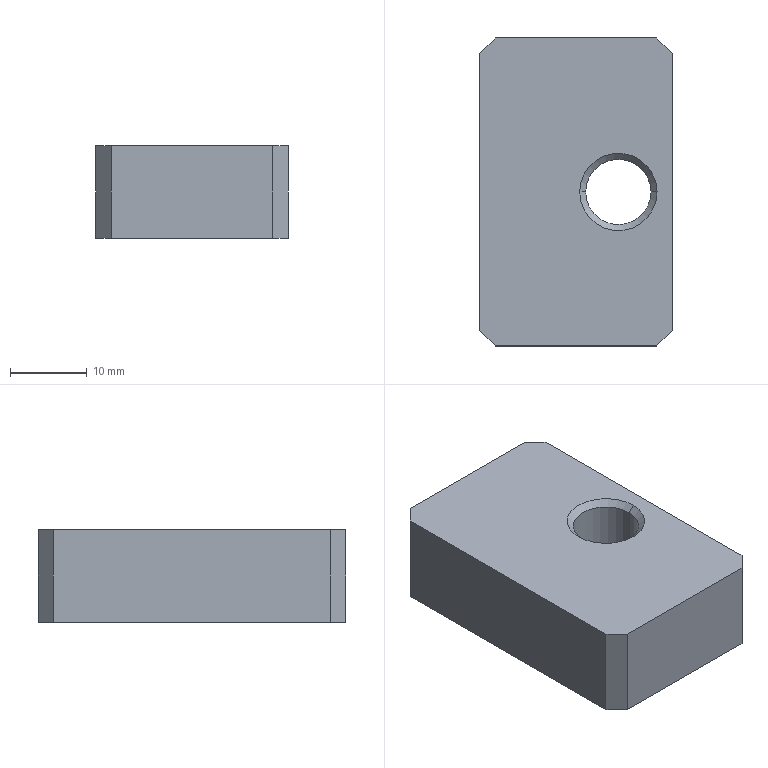Part | STEP file | 001-004-Feeding mechanism hydraulic buffer mounting plate | 1 solid | 14 faces | box 25 x 40 x 12 mm | volume 11215 mm3 | plane 10 | cone 2 | cylinder 2 | commonest cylinder face diameters 8.5 x2
STEP:
#1=CARTESIAN_POINT('',(0.,0.,0.));
#2=DIRECTION('',(0.,0.,1.));
#3=DIRECTION('',(1.,0.,0.));
#4=AXIS2_PLACEMENT_3D('',#1,#2,#3);
#5=CARTESIAN_POINT('',(9.75,0.,11.225));
#6=VERTEX_POINT('',#5);
#7=CARTESIAN_POINT('',(10.525,0.,12.));
#8=VERTEX_POINT('',#7);
#9=CARTESIAN_POINT('',(10.525,0.,12.));
#10=DIRECTION('',(0.7071,0.,0.7071));
#11=VECTOR('',#10,1.);
#12=LINE('',#9,#11);
#13=CARTESIAN_POINT('',(5.5,0.,12.));
#14=DIRECTION('',(0.,0.,1.));
#15=DIRECTION('',(1.,0.,0.));
#16=AXIS2_PLACEMENT_3D('',#13,#14,#15);
#17=CONICAL_SURFACE('',#16,5.025,0.7854);
#18=CARTESIAN_POINT('',(6.283,0.));
#19=DIRECTION('',(0.,1.));
#20=VECTOR('',#19,1.);
#21=LINE('',#18,#20);
#22=(GEOMETRIC_REPRESENTATION_CONTEXT(2)PARAMETRIC_REPRESENTATION_CONTEXT()REPRESENTATION_CONTEXT('',''));
#23=DEFINITIONAL_REPRESENTATION('',(#21),#22);
#24=PCURVE('',#17,#23);
#25=CARTESIAN_POINT('',(5.5,0.,12.));
#26=DIRECTION('',(0.,0.,1.));
#27=DIRECTION('',(1.,0.,0.));
#28=AXIS2_PLACEMENT_3D('',#25,#26,#27);
#29=CONICAL_SURFACE('',#28,5.025,0.7854);
#30=CARTESIAN_POINT('',(0.,0.));
#31=DIRECTION('',(0.,1.));
#32=VECTOR('',#31,1.);
#33=LINE('',#30,#32);
#34=(GEOMETRIC_REPRESENTATION_CONTEXT(2)PARAMETRIC_REPRESENTATION_CONTEXT()REPRESENTATION_CONTEXT('',''));
#35=DEFINITIONAL_REPRESENTATION('',(#33),#34);
#36=PCURVE('',#29,#35);
#37=SURFACE_CURVE('',#12,(#24,#36),.PCURVE_S1.);
#38=EDGE_CURVE('',#6,#8,#37,.T.);
#39=ORIENTED_EDGE('',*,*,#38,.T.);
#40=CARTESIAN_POINT('',(0.475,0.,12.));
#41=VERTEX_POINT('',#40);
#42=CARTESIAN_POINT('',(5.5,0.,12.));
#43=DIRECTION('',(0.,0.,1.));
#44=DIRECTION('',(1.,0.,0.));
#45=AXIS2_PLACEMENT_3D('',#42,#43,#44);
#46=CIRCLE('',#45,5.025);
#47=CARTESIAN_POINT('',(0.,0.));
#48=DIRECTION('',(1.,0.));
#49=VECTOR('',#48,1.);
#50=LINE('',#47,#49);
#51=(GEOMETRIC_REPRESENTATION_CONTEXT(2)PARAMETRIC_REPRESENTATION_CONTEXT()REPRESENTATION_CONTEXT('',''));
#52=DEFINITIONAL_REPRESENTATION('',(#50),#51);
#53=PCURVE('',#17,#52);
#54=CARTESIAN_POINT('',(0.,0.,12.));
#55=DIRECTION('',(0.,0.,-1.));
#56=DIRECTION('',(-1.,0.,0.));
#57=AXIS2_PLACEMENT_3D('',#54,#55,#56);
#58=PLANE('',#57);
#59=CARTESIAN_POINT('',(-10.525,0.));
#60=CARTESIAN_POINT('',(-10.525,8.704));
#61=CARTESIAN_POINT('',(-2.988,4.352));
#62=CARTESIAN_POINT('',(4.55,0.));
#63=CARTESIAN_POINT('',(-2.988,-4.352));
#64=CARTESIAN_POINT('',(-10.525,-8.704));
#65=CARTESIAN_POINT('',(-10.525,0.));
#66=(BOUNDED_CURVE()B_SPLINE_CURVE(2,(#59,#60,#61,#62,#63,#64,#65),.UNSPECIFIED.,.T.,.F.)B_SPLINE_CURVE_WITH_KNOTS((1,2,2,2,2,1),(-2.094,0.,2.094,4.189,6.283,8.378),.UNSPECIFIED.)CURVE()GEOMETRIC_REPRESENTATION_ITEM()RATIONAL_B_SPLINE_CURVE((1.,0.5,1.,0.5,1.,0.5,1.))REPRESENTATION_ITEM(''));
#67=(GEOMETRIC_REPRESENTATION_CONTEXT(2)PARAMETRIC_REPRESENTATION_CONTEXT()REPRESENTATION_CONTEXT('',''));
#68=DEFINITIONAL_REPRESENTATION('',(#66),#67);
#69=PCURVE('',#58,#68);
#70=SURFACE_CURVE('',#46,(#53,#69),.PCURVE_S1.);
#71=EDGE_CURVE('',#41,#8,#70,.T.);
#72=ORIENTED_EDGE('',*,*,#71,.F.);
#73=CARTESIAN_POINT('',(1.25,0.,11.225));
#74=VERTEX_POINT('',#73);
#75=CARTESIAN_POINT('',(0.475,0.,12.));
#76=DIRECTION('',(-0.7071,0.,0.7071));
#77=VECTOR('',#76,1.);
#78=LINE('',#75,#77);
#79=CARTESIAN_POINT('',(3.142,0.));
#80=DIRECTION('',(0.,1.));
#81=VECTOR('',#80,1.);
#82=LINE('',#79,#81);
#83=(GEOMETRIC_REPRESENTATION_CONTEXT(2)PARAMETRIC_REPRESENTATION_CONTEXT()REPRESENTATION_CONTEXT('',''));
#84=DEFINITIONAL_REPRESENTATION('',(#82),#83);
#85=PCURVE('',#17,#84);
#86=CARTESIAN_POINT('',(3.142,0.));
#87=DIRECTION('',(0.,1.));
#88=VECTOR('',#87,1.);
#89=LINE('',#86,#88);
#90=(GEOMETRIC_REPRESENTATION_CONTEXT(2)PARAMETRIC_REPRESENTATION_CONTEXT()REPRESENTATION_CONTEXT('',''));
#91=DEFINITIONAL_REPRESENTATION('',(#89),#90);
#92=PCURVE('',#29,#91);
#93=SURFACE_CURVE('',#78,(#85,#92),.PCURVE_S1.);
#94=EDGE_CURVE('',#74,#41,#93,.T.);
#95=ORIENTED_EDGE('',*,*,#94,.F.);
#96=CARTESIAN_POINT('',(5.5,0.,11.225));
#97=DIRECTION('',(0.,0.,1.));
#98=DIRECTION('',(1.,0.,0.));
#99=AXIS2_PLACEMENT_3D('',#96,#97,#98);
#100=CIRCLE('',#99,4.25);
#101=CARTESIAN_POINT('',(0.,-0.775));
#102=DIRECTION('',(1.,0.));
#103=VECTOR('',#102,1.);
#104=LINE('',#101,#103);
#105=(GEOMETRIC_REPRESENTATION_CONTEXT(2)PARAMETRIC_REPRESENTATION_CONTEXT()REPRESENTATION_CONTEXT('',''));
#106=DEFINITIONAL_REPRESENTATION('',(#104),#105);
#107=PCURVE('',#17,#106);
#108=CARTESIAN_POINT('',(5.5,0.,12.));
#109=DIRECTION('',(0.,0.,1.));
#110=DIRECTION('',(1.,0.,0.));
#111=AXIS2_PLACEMENT_3D('',#108,#109,#110);
#112=CYLINDRICAL_SURFACE('',#111,4.25);
#113=CARTESIAN_POINT('',(0.,-0.775));
#114=DIRECTION('',(1.,0.));
#115=VECTOR('',#114,1.);
#116=LINE('',#113,#115);
#117=(GEOMETRIC_REPRESENTATION_CONTEXT(2)PARAMETRIC_REPRESENTATION_CONTEXT()REPRESENTATION_CONTEXT('',''));
#118=DEFINITIONAL_REPRESENTATION('',(#116),#117);
#119=PCURVE('',#112,#118);
#120=SURFACE_CURVE('',#100,(#107,#119),.PCURVE_S1.);
#121=EDGE_CURVE('',#74,#6,#120,.T.);
#122=ORIENTED_EDGE('',*,*,#121,.T.);
#123=EDGE_LOOP('',(#39,#72,#95,#122));
#124=FACE_BOUND('',#123,.F.);
#125=ADVANCED_FACE('',(#124),#17,.F.);
#126=CARTESIAN_POINT('',(9.75,0.,0.));
#127=VERTEX_POINT('',#126);
#128=CARTESIAN_POINT('',(9.75,0.,12.));
#129=DIRECTION('',(0.,0.,1.));
#130=VECTOR('',#129,1.);
#131=LINE('',#128,#130);
#132=CARTESIAN_POINT('',(6.283,0.));
#133=DIRECTION('',(0.,1.));
#134=VECTOR('',#133,1.);
#135=LINE('',#132,#134);
#136=(GEOMETRIC_REPRESENTATION_CONTEXT(2)PARAMETRIC_REPRESENTATION_CONTEXT()REPRESENTATION_CONTEXT('',''));
#137=DEFINITIONAL_REPRESENTATION('',(#135),#136);
#138=PCURVE('',#112,#137);
#139=CARTESIAN_POINT('',(5.5,0.,12.));
#140=DIRECTION('',(0.,0.,1.));
#141=DIRECTION('',(1.,0.,0.));
#142=AXIS2_PLACEMENT_3D('',#139,#140,#141);
#143=CYLINDRICAL_SURFACE('',#142,4.25);
#144=CARTESIAN_POINT('',(0.,0.));
#145=DIRECTION('',(0.,1.));
#146=VECTOR('',#145,1.);
#147=LINE('',#144,#146);
#148=(GEOMETRIC_REPRESENTATION_CONTEXT(2)PARAMETRIC_REPRESENTATION_CONTEXT()REPRESENTATION_CONTEXT('',''));
#149=DEFINITIONAL_REPRESENTATION('',(#147),#148);
#150=PCURVE('',#143,#149);
#151=SURFACE_CURVE('',#131,(#138,#150),.PCURVE_S1.);
#152=EDGE_CURVE('',#127,#6,#151,.T.);
#153=ORIENTED_EDGE('',*,*,#152,.T.);
#154=ORIENTED_EDGE('',*,*,#121,.F.);
#155=CARTESIAN_POINT('',(1.25,0.,0.));
#156=VERTEX_POINT('',#155);
#157=CARTESIAN_POINT('',(1.25,0.,12.));
#158=DIRECTION('',(0.,0.,1.));
#159=VECTOR('',#158,1.);
#160=LINE('',#157,#159);
#161=CARTESIAN_POINT('',(3.142,0.));
#162=DIRECTION('',(0.,1.));
#163=VECTOR('',#162,1.);
#164=LINE('',#161,#163);
#165=(GEOMETRIC_REPRESENTATION_CONTEXT(2)PARAMETRIC_REPRESENTATION_CONTEXT()REPRESENTATION_CONTEXT('',''));
#166=DEFINITIONAL_REPRESENTATION('',(#164),#165);
#167=PCURVE('',#112,#166);
#168=CARTESIAN_POINT('',(3.142,0.));
#169=DIRECTION('',(0.,1.));
#170=VECTOR('',#169,1.);
#171=LINE('',#168,#170);
#172=(GEOMETRIC_REPRESENTATION_CONTEXT(2)PARAMETRIC_REPRESENTATION_CONTEXT()REPRESENTATION_CONTEXT('',''));
#173=DEFINITIONAL_REPRESENTATION('',(#171),#172);
#174=PCURVE('',#143,#173);
#175=SURFACE_CURVE('',#160,(#167,#174),.PCURVE_S1.);
#176=EDGE_CURVE('',#156,#74,#175,.T.);
#177=ORIENTED_EDGE('',*,*,#176,.F.);
#178=CARTESIAN_POINT('',(5.5,0.,0.));
#179=DIRECTION('',(0.,0.,1.));
#180=DIRECTION('',(1.,0.,0.));
#181=AXIS2_PLACEMENT_3D('',#178,#179,#180);
#182=CIRCLE('',#181,4.25);
#183=CARTESIAN_POINT('',(0.,-12.));
#184=DIRECTION('',(1.,0.));
#185=VECTOR('',#184,1.);
#186=LINE('',#183,#185);
#187=(GEOMETRIC_REPRESENTATION_CONTEXT(2)PARAMETRIC_REPRESENTATION_CONTEXT()REPRESENTATION_CONTEXT('',''));
#188=DEFINITIONAL_REPRESENTATION('',(#186),#187);
#189=PCURVE('',#112,#188);
#190=CARTESIAN_POINT('',(0.,0.,0.));
#191=DIRECTION('',(0.,0.,-1.));
#192=DIRECTION('',(-1.,0.,0.));
#193=AXIS2_PLACEMENT_3D('',#190,#191,#192);
#194=PLANE('',#193);
#195=CARTESIAN_POINT('',(-9.75,0.));
#196=CARTESIAN_POINT('',(-9.75,7.361));
#197=CARTESIAN_POINT('',(-3.375,3.681));
#198=CARTESIAN_POINT('',(3.,0.));
#199=CARTESIAN_POINT('',(-3.375,-3.681));
#200=CARTESIAN_POINT('',(-9.75,-7.361));
#201=CARTESIAN_POINT('',(-9.75,0.));
#202=(BOUNDED_CURVE()B_SPLINE_CURVE(2,(#195,#196,#197,#198,#199,#200,#201),.UNSPECIFIED.,.T.,.F.)B_SPLINE_CURVE_WITH_KNOTS((1,2,2,2,2,1),(-2.094,0.,2.094,4.189,6.283,8.378),.UNSPECIFIED.)CURVE()GEOMETRIC_REPRESENTATION_ITEM()RATIONAL_B_SPLINE_CURVE((1.,0.5,1.,0.5,1.,0.5,1.))REPRESENTATION_ITEM(''));
#203=(GEOMETRIC_REPRESENTATION_CONTEXT(2)PARAMETRIC_REPRESENTATION_CONTEXT()REPRESENTATION_CONTEXT('',''));
#204=DEFINITIONAL_REPRESENTATION('',(#202),#203);
#205=PCURVE('',#194,#204);
#206=SURFACE_CURVE('',#182,(#189,#205),.PCURVE_S1.);
#207=EDGE_CURVE('',#156,#127,#206,.T.);
#208=ORIENTED_EDGE('',*,*,#207,.T.);
#209=EDGE_LOOP('',(#153,#154,#177,#208));
#210=FACE_BOUND('',#209,.F.);
#211=ADVANCED_FACE('',(#210),#112,.F.);
#212=CARTESIAN_POINT('',(12.5,-18.,12.));
#213=VERTEX_POINT('',#212);
#214=CARTESIAN_POINT('',(12.5,18.,12.));
#215=VERTEX_POINT('',#214);
#216=CARTESIAN_POINT('',(12.5,-20.,12.));
#217=DIRECTION('',(0.,1.,0.));
#218=VECTOR('',#217,1.);
#219=LINE('',#216,#218);
#220=CARTESIAN_POINT('',(12.5,-20.,12.));
#221=DIRECTION('',(-1.,0.,0.));
#222=DIRECTION('',(0.,0.,1.));
#223=AXIS2_PLACEMENT_3D('',#220,#221,#222);
#224=PLANE('',#223);
#225=CARTESIAN_POINT('',(0.,0.));
#226=DIRECTION('',(0.,1.));
#227=VECTOR('',#226,1.);
#228=LINE('',#225,#227);
#229=(GEOMETRIC_REPRESENTATION_CONTEXT(2)PARAMETRIC_REPRESENTATION_CONTEXT()REPRESENTATION_CONTEXT('',''));
#230=DEFINITIONAL_REPRESENTATION('',(#228),#229);
#231=PCURVE('',#224,#230);
#232=CARTESIAN_POINT('',(-12.5,-20.));
#233=DIRECTION('',(0.,1.));
#234=VECTOR('',#233,1.);
#235=LINE('',#232,#234);
#236=(GEOMETRIC_REPRESENTATION_CONTEXT(2)PARAMETRIC_REPRESENTATION_CONTEXT()REPRESENTATION_CONTEXT('',''));
#237=DEFINITIONAL_REPRESENTATION('',(#235),#236);
#238=PCURVE('',#58,#237);
#239=SURFACE_CURVE('',#219,(#231,#238),.PCURVE_S1.);
#240=EDGE_CURVE('',#213,#215,#239,.T.);
#241=ORIENTED_EDGE('',*,*,#240,.F.);
#242=CARTESIAN_POINT('',(12.5,-18.,0.));
#243=VERTEX_POINT('',#242);
#244=CARTESIAN_POINT('',(12.5,-18.,12.));
#245=DIRECTION('',(0.,0.,-1.));
#246=VECTOR('',#245,1.);
#247=LINE('',#244,#246);
#248=CARTESIAN_POINT('',(0.,2.));
#249=DIRECTION('',(-1.,0.));
#250=VECTOR('',#249,1.);
#251=LINE('',#248,#250);
#252=(GEOMETRIC_REPRESENTATION_CONTEXT(2)PARAMETRIC_REPRESENTATION_CONTEXT()REPRESENTATION_CONTEXT('',''));
#253=DEFINITIONAL_REPRESENTATION('',(#251),#252);
#254=PCURVE('',#224,#253);
#255=CARTESIAN_POINT('',(12.5,-18.,12.));
#256=DIRECTION('',(-0.7071,0.7071,0.));
#257=DIRECTION('',(0.,0.,-1.));
#258=AXIS2_PLACEMENT_3D('',#255,#256,#257);
#259=PLANE('',#258);
#260=CARTESIAN_POINT('',(0.,0.));
#261=DIRECTION('',(1.,0.));
#262=VECTOR('',#261,1.);
#263=LINE('',#260,#262);
#264=(GEOMETRIC_REPRESENTATION_CONTEXT(2)PARAMETRIC_REPRESENTATION_CONTEXT()REPRESENTATION_CONTEXT('',''));
#265=DEFINITIONAL_REPRESENTATION('',(#263),#264);
#266=PCURVE('',#259,#265);
#267=SURFACE_CURVE('',#247,(#254,#266),.PCURVE_S1.);
#268=EDGE_CURVE('',#213,#243,#267,.T.);
#269=ORIENTED_EDGE('',*,*,#268,.T.);
#270=CARTESIAN_POINT('',(12.5,18.,0.));
#271=VERTEX_POINT('',#270);
#272=CARTESIAN_POINT('',(12.5,-20.,0.));
#273=DIRECTION('',(0.,1.,0.));
#274=VECTOR('',#273,1.);
#275=LINE('',#272,#274);
#276=CARTESIAN_POINT('',(-12.,0.));
#277=DIRECTION('',(0.,1.));
#278=VECTOR('',#277,1.);
#279=LINE('',#276,#278);
#280=(GEOMETRIC_REPRESENTATION_CONTEXT(2)PARAMETRIC_REPRESENTATION_CONTEXT()REPRESENTATION_CONTEXT('',''));
#281=DEFINITIONAL_REPRESENTATION('',(#279),#280);
#282=PCURVE('',#224,#281);
#283=CARTESIAN_POINT('',(-12.5,-20.));
#284=DIRECTION('',(0.,1.));
#285=VECTOR('',#284,1.);
#286=LINE('',#283,#285);
#287=(GEOMETRIC_REPRESENTATION_CONTEXT(2)PARAMETRIC_REPRESENTATION_CONTEXT()REPRESENTATION_CONTEXT('',''));
#288=DEFINITIONAL_REPRESENTATION('',(#286),#287);
#289=PCURVE('',#194,#288);
#290=SURFACE_CURVE('',#275,(#282,#289),.PCURVE_S1.);
#291=EDGE_CURVE('',#243,#271,#290,.T.);
#292=ORIENTED_EDGE('',*,*,#291,.T.);
#293=CARTESIAN_POINT('',(12.5,18.,12.));
#294=DIRECTION('',(0.,0.,1.));
#295=VECTOR('',#294,1.);
#296=LINE('',#293,#295);
#297=CARTESIAN_POINT('',(0.,38.));
#298=DIRECTION('',(1.,0.));
#299=VECTOR('',#298,1.);
#300=LINE('',#297,#299);
#301=(GEOMETRIC_REPRESENTATION_CONTEXT(2)PARAMETRIC_REPRESENTATION_CONTEXT()REPRESENTATION_CONTEXT('',''));
#302=DEFINITIONAL_REPRESENTATION('',(#300),#301);
#303=PCURVE('',#224,#302);
#304=CARTESIAN_POINT('',(10.5,20.,12.));
#305=DIRECTION('',(-0.7071,-0.7071,0.));
#306=DIRECTION('',(0.,0.,-1.));
#307=AXIS2_PLACEMENT_3D('',#304,#305,#306);
#308=PLANE('',#307);
#309=CARTESIAN_POINT('',(0.,2.828));
#310=DIRECTION('',(-1.,0.));
#311=VECTOR('',#310,1.);
#312=LINE('',#309,#311);
#313=(GEOMETRIC_REPRESENTATION_CONTEXT(2)PARAMETRIC_REPRESENTATION_CONTEXT()REPRESENTATION_CONTEXT('',''));
#314=DEFINITIONAL_REPRESENTATION('',(#312),#313);
#315=PCURVE('',#308,#314);
#316=SURFACE_CURVE('',#296,(#303,#315),.PCURVE_S1.);
#317=EDGE_CURVE('',#271,#215,#316,.T.);
#318=ORIENTED_EDGE('',*,*,#317,.T.);
#319=EDGE_LOOP('',(#241,#269,#292,#318));
#320=FACE_BOUND('',#319,.T.);
#321=ADVANCED_FACE('',(#320),#224,.F.);
#322=CARTESIAN_POINT('',(10.5,20.,0.));
#323=VERTEX_POINT('',#322);
#324=CARTESIAN_POINT('',(-10.5,20.,0.));
#325=VERTEX_POINT('',#324);
#326=CARTESIAN_POINT('',(-12.5,20.,0.));
#327=DIRECTION('',(-1.,0.,0.));
#328=VECTOR('',#327,1.);
#329=LINE('',#326,#328);
#330=CARTESIAN_POINT('',(-12.5,20.,12.));
#331=DIRECTION('',(0.,-1.,0.));
#332=DIRECTION('',(0.,0.,-1.));
#333=AXIS2_PLACEMENT_3D('',#330,#331,#332);
#334=PLANE('',#333);
#335=CARTESIAN_POINT('',(12.,0.));
#336=DIRECTION('',(0.,-1.));
#337=VECTOR('',#336,1.);
#338=LINE('',#335,#337);
#339=(GEOMETRIC_REPRESENTATION_CONTEXT(2)PARAMETRIC_REPRESENTATION_CONTEXT()REPRESENTATION_CONTEXT('',''));
#340=DEFINITIONAL_REPRESENTATION('',(#338),#339);
#341=PCURVE('',#334,#340);
#342=CARTESIAN_POINT('',(12.5,20.));
#343=DIRECTION('',(1.,0.));
#344=VECTOR('',#343,1.);
#345=LINE('',#342,#344);
#346=(GEOMETRIC_REPRESENTATION_CONTEXT(2)PARAMETRIC_REPRESENTATION_CONTEXT()REPRESENTATION_CONTEXT('',''));
#347=DEFINITIONAL_REPRESENTATION('',(#345),#346);
#348=PCURVE('',#194,#347);
#349=SURFACE_CURVE('',#329,(#341,#348),.PCURVE_S1.);
#350=EDGE_CURVE('',#323,#325,#349,.T.);
#351=ORIENTED_EDGE('',*,*,#350,.T.);
#352=CARTESIAN_POINT('',(-10.5,20.,12.));
#353=VERTEX_POINT('',#352);
#354=CARTESIAN_POINT('',(-10.5,20.,12.));
#355=DIRECTION('',(0.,0.,1.));
#356=VECTOR('',#355,1.);
#357=LINE('',#354,#356);
#358=CARTESIAN_POINT('',(0.,2.));
#359=DIRECTION('',(-1.,0.));
#360=VECTOR('',#359,1.);
#361=LINE('',#358,#360);
#362=(GEOMETRIC_REPRESENTATION_CONTEXT(2)PARAMETRIC_REPRESENTATION_CONTEXT()REPRESENTATION_CONTEXT('',''));
#363=DEFINITIONAL_REPRESENTATION('',(#361),#362);
#364=PCURVE('',#334,#363);
#365=CARTESIAN_POINT('',(-12.5,18.,12.));
#366=DIRECTION('',(0.7071,-0.7071,0.));
#367=DIRECTION('',(0.,0.,-1.));
#368=AXIS2_PLACEMENT_3D('',#365,#366,#367);
#369=PLANE('',#368);
#370=CARTESIAN_POINT('',(0.,2.828));
#371=DIRECTION('',(-1.,0.));
#372=VECTOR('',#371,1.);
#373=LINE('',#370,#372);
#374=(GEOMETRIC_REPRESENTATION_CONTEXT(2)PARAMETRIC_REPRESENTATION_CONTEXT()REPRESENTATION_CONTEXT('',''));
#375=DEFINITIONAL_REPRESENTATION('',(#373),#374);
#376=PCURVE('',#369,#375);
#377=SURFACE_CURVE('',#357,(#364,#376),.PCURVE_S1.);
#378=EDGE_CURVE('',#325,#353,#377,.T.);
#379=ORIENTED_EDGE('',*,*,#378,.T.);
#380=CARTESIAN_POINT('',(10.5,20.,12.));
#381=VERTEX_POINT('',#380);
#382=CARTESIAN_POINT('',(-12.5,20.,12.));
#383=DIRECTION('',(-1.,0.,0.));
#384=VECTOR('',#383,1.);
#385=LINE('',#382,#384);
#386=CARTESIAN_POINT('',(0.,0.));
#387=DIRECTION('',(0.,-1.));
#388=VECTOR('',#387,1.);
#389=LINE('',#386,#388);
#390=(GEOMETRIC_REPRESENTATION_CONTEXT(2)PARAMETRIC_REPRESENTATION_CONTEXT()REPRESENTATION_CONTEXT('',''));
#391=DEFINITIONAL_REPRESENTATION('',(#389),#390);
#392=PCURVE('',#334,#391);
#393=CARTESIAN_POINT('',(12.5,20.));
#394=DIRECTION('',(1.,0.));
#395=VECTOR('',#394,1.);
#396=LINE('',#393,#395);
#397=(GEOMETRIC_REPRESENTATION_CONTEXT(2)PARAMETRIC_REPRESENTATION_CONTEXT()REPRESENTATION_CONTEXT('',''));
#398=DEFINITIONAL_REPRESENTATION('',(#396),#397);
#399=PCURVE('',#58,#398);
#400=SURFACE_CURVE('',#385,(#392,#399),.PCURVE_S1.);
#401=EDGE_CURVE('',#381,#353,#400,.T.);
#402=ORIENTED_EDGE('',*,*,#401,.F.);
#403=CARTESIAN_POINT('',(10.5,20.,12.));
#404=DIRECTION('',(0.,0.,-1.));
#405=VECTOR('',#404,1.);
#406=LINE('',#403,#405);
#407=CARTESIAN_POINT('',(0.,23.));
#408=DIRECTION('',(1.,0.));
#409=VECTOR('',#408,1.);
#410=LINE('',#407,#409);
#411=(GEOMETRIC_REPRESENTATION_CONTEXT(2)PARAMETRIC_REPRESENTATION_CONTEXT()REPRESENTATION_CONTEXT('',''));
#412=DEFINITIONAL_REPRESENTATION('',(#410),#411);
#413=PCURVE('',#334,#412);
#414=CARTESIAN_POINT('',(0.,0.));
#415=DIRECTION('',(1.,0.));
#416=VECTOR('',#415,1.);
#417=LINE('',#414,#416);
#418=(GEOMETRIC_REPRESENTATION_CONTEXT(2)PARAMETRIC_REPRESENTATION_CONTEXT()REPRESENTATION_CONTEXT('',''));
#419=DEFINITIONAL_REPRESENTATION('',(#417),#418);
#420=PCURVE('',#308,#419);
#421=SURFACE_CURVE('',#406,(#413,#420),.PCURVE_S1.);
#422=EDGE_CURVE('',#381,#323,#421,.T.);
#423=ORIENTED_EDGE('',*,*,#422,.T.);
#424=EDGE_LOOP('',(#351,#379,#402,#423));
#425=FACE_BOUND('',#424,.T.);
#426=ADVANCED_FACE('',(#425),#334,.F.);
#427=CARTESIAN_POINT('',(-12.5,18.,0.));
#428=VERTEX_POINT('',#427);
#429=CARTESIAN_POINT('',(-12.5,-18.,0.));
#430=VERTEX_POINT('',#429);
#431=CARTESIAN_POINT('',(-12.5,-20.,0.));
#432=DIRECTION('',(0.,-1.,0.));
#433=VECTOR('',#432,1.);
#434=LINE('',#431,#433);
#435=CARTESIAN_POINT('',(-12.5,-20.,12.));
#436=DIRECTION('',(1.,0.,0.));
#437=DIRECTION('',(0.,0.,-1.));
#438=AXIS2_PLACEMENT_3D('',#435,#436,#437);
#439=PLANE('',#438);
#440=CARTESIAN_POINT('',(12.,0.));
#441=DIRECTION('',(0.,-1.));
#442=VECTOR('',#441,1.);
#443=LINE('',#440,#442);
#444=(GEOMETRIC_REPRESENTATION_CONTEXT(2)PARAMETRIC_REPRESENTATION_CONTEXT()REPRESENTATION_CONTEXT('',''));
#445=DEFINITIONAL_REPRESENTATION('',(#443),#444);
#446=PCURVE('',#439,#445);
#447=CARTESIAN_POINT('',(12.5,-20.));
#448=DIRECTION('',(0.,-1.));
#449=VECTOR('',#448,1.);
#450=LINE('',#447,#449);
#451=(GEOMETRIC_REPRESENTATION_CONTEXT(2)PARAMETRIC_REPRESENTATION_CONTEXT()REPRESENTATION_CONTEXT('',''));
#452=DEFINITIONAL_REPRESENTATION('',(#450),#451);
#453=PCURVE('',#194,#452);
#454=SURFACE_CURVE('',#434,(#446,#453),.PCURVE_S1.);
#455=EDGE_CURVE('',#428,#430,#454,.T.);
#456=ORIENTED_EDGE('',*,*,#455,.T.);
#457=CARTESIAN_POINT('',(-12.5,-18.,12.));
#458=VERTEX_POINT('',#457);
#459=CARTESIAN_POINT('',(-12.5,-18.,12.));
#460=DIRECTION('',(0.,0.,1.));
#461=VECTOR('',#460,1.);
#462=LINE('',#459,#461);
#463=CARTESIAN_POINT('',(0.,2.));
#464=DIRECTION('',(-1.,0.));
#465=VECTOR('',#464,1.);
#466=LINE('',#463,#465);
#467=(GEOMETRIC_REPRESENTATION_CONTEXT(2)PARAMETRIC_REPRESENTATION_CONTEXT()REPRESENTATION_CONTEXT('',''));
#468=DEFINITIONAL_REPRESENTATION('',(#466),#467);
#469=PCURVE('',#439,#468);
#470=CARTESIAN_POINT('',(-10.5,-20.,12.));
#471=DIRECTION('',(0.7071,0.7071,0.));
#472=DIRECTION('',(0.,0.,-1.));
#473=AXIS2_PLACEMENT_3D('',#470,#471,#472);
#474=PLANE('',#473);
#475=CARTESIAN_POINT('',(0.,2.828));
#476=DIRECTION('',(-1.,0.));
#477=VECTOR('',#476,1.);
#478=LINE('',#475,#477);
#479=(GEOMETRIC_REPRESENTATION_CONTEXT(2)PARAMETRIC_REPRESENTATION_CONTEXT()REPRESENTATION_CONTEXT('',''));
#480=DEFINITIONAL_REPRESENTATION('',(#478),#479);
#481=PCURVE('',#474,#480);
#482=SURFACE_CURVE('',#462,(#469,#481),.PCURVE_S1.);
#483=EDGE_CURVE('',#430,#458,#482,.T.);
#484=ORIENTED_EDGE('',*,*,#483,.T.);
#485=CARTESIAN_POINT('',(-12.5,18.,12.));
#486=VERTEX_POINT('',#485);
#487=CARTESIAN_POINT('',(-12.5,-20.,12.));
#488=DIRECTION('',(0.,-1.,0.));
#489=VECTOR('',#488,1.);
#490=LINE('',#487,#489);
#491=CARTESIAN_POINT('',(0.,0.));
#492=DIRECTION('',(0.,-1.));
#493=VECTOR('',#492,1.);
#494=LINE('',#491,#493);
#495=(GEOMETRIC_REPRESENTATION_CONTEXT(2)PARAMETRIC_REPRESENTATION_CONTEXT()REPRESENTATION_CONTEXT('',''));
#496=DEFINITIONAL_REPRESENTATION('',(#494),#495);
#497=PCURVE('',#439,#496);
#498=CARTESIAN_POINT('',(12.5,-20.));
#499=DIRECTION('',(0.,-1.));
#500=VECTOR('',#499,1.);
#501=LINE('',#498,#500);
#502=(GEOMETRIC_REPRESENTATION_CONTEXT(2)PARAMETRIC_REPRESENTATION_CONTEXT()REPRESENTATION_CONTEXT('',''));
#503=DEFINITIONAL_REPRESENTATION('',(#501),#502);
#504=PCURVE('',#58,#503);
#505=SURFACE_CURVE('',#490,(#497,#504),.PCURVE_S1.);
#506=EDGE_CURVE('',#486,#458,#505,.T.);
#507=ORIENTED_EDGE('',*,*,#506,.F.);
#508=CARTESIAN_POINT('',(-12.5,18.,12.));
#509=DIRECTION('',(0.,0.,-1.));
#510=VECTOR('',#509,1.);
#511=LINE('',#508,#510);
#512=CARTESIAN_POINT('',(0.,38.));
#513=DIRECTION('',(1.,0.));
#514=VECTOR('',#513,1.);
#515=LINE('',#512,#514);
#516=(GEOMETRIC_REPRESENTATION_CONTEXT(2)PARAMETRIC_REPRESENTATION_CONTEXT()REPRESENTATION_CONTEXT('',''));
#517=DEFINITIONAL_REPRESENTATION('',(#515),#516);
#518=PCURVE('',#439,#517);
#519=CARTESIAN_POINT('',(0.,0.));
#520=DIRECTION('',(1.,0.));
#521=VECTOR('',#520,1.);
#522=LINE('',#519,#521);
#523=(GEOMETRIC_REPRESENTATION_CONTEXT(2)PARAMETRIC_REPRESENTATION_CONTEXT()REPRESENTATION_CONTEXT('',''));
#524=DEFINITIONAL_REPRESENTATION('',(#522),#523);
#525=PCURVE('',#369,#524);
#526=SURFACE_CURVE('',#511,(#518,#525),.PCURVE_S1.);
#527=EDGE_CURVE('',#486,#428,#526,.T.);
#528=ORIENTED_EDGE('',*,*,#527,.T.);
#529=EDGE_LOOP('',(#456,#484,#507,#528));
#530=FACE_BOUND('',#529,.T.);
#531=ADVANCED_FACE('',(#530),#439,.F.);
#532=CARTESIAN_POINT('',(-10.5,-20.,0.));
#533=VERTEX_POINT('',#532);
#534=CARTESIAN_POINT('',(10.5,-20.,0.));
#535=VERTEX_POINT('',#534);
#536=CARTESIAN_POINT('',(-12.5,-20.,0.));
#537=DIRECTION('',(1.,0.,0.));
#538=VECTOR('',#537,1.);
#539=LINE('',#536,#538);
#540=CARTESIAN_POINT('',(-12.5,-20.,12.));
#541=DIRECTION('',(0.,1.,0.));
#542=DIRECTION('',(0.,0.,1.));
#543=AXIS2_PLACEMENT_3D('',#540,#541,#542);
#544=PLANE('',#543);
#545=CARTESIAN_POINT('',(-12.,0.));
#546=DIRECTION('',(0.,1.));
#547=VECTOR('',#546,1.);
#548=LINE('',#545,#547);
#549=(GEOMETRIC_REPRESENTATION_CONTEXT(2)PARAMETRIC_REPRESENTATION_CONTEXT()REPRESENTATION_CONTEXT('',''));
#550=DEFINITIONAL_REPRESENTATION('',(#548),#549);
#551=PCURVE('',#544,#550);
#552=CARTESIAN_POINT('',(12.5,-20.));
#553=DIRECTION('',(-1.,0.));
#554=VECTOR('',#553,1.);
#555=LINE('',#552,#554);
#556=(GEOMETRIC_REPRESENTATION_CONTEXT(2)PARAMETRIC_REPRESENTATION_CONTEXT()REPRESENTATION_CONTEXT('',''));
#557=DEFINITIONAL_REPRESENTATION('',(#555),#556);
#558=PCURVE('',#194,#557);
#559=SURFACE_CURVE('',#539,(#551,#558),.PCURVE_S1.);
#560=EDGE_CURVE('',#533,#535,#559,.T.);
#561=ORIENTED_EDGE('',*,*,#560,.T.);
#562=CARTESIAN_POINT('',(10.5,-20.,12.));
#563=VERTEX_POINT('',#562);
#564=CARTESIAN_POINT('',(10.5,-20.,12.));
#565=DIRECTION('',(0.,0.,1.));
#566=VECTOR('',#565,1.);
#567=LINE('',#564,#566);
#568=CARTESIAN_POINT('',(0.,23.));
#569=DIRECTION('',(1.,0.));
#570=VECTOR('',#569,1.);
#571=LINE('',#568,#570);
#572=(GEOMETRIC_REPRESENTATION_CONTEXT(2)PARAMETRIC_REPRESENTATION_CONTEXT()REPRESENTATION_CONTEXT('',''));
#573=DEFINITIONAL_REPRESENTATION('',(#571),#572);
#574=PCURVE('',#544,#573);
#575=CARTESIAN_POINT('',(0.,2.828));
#576=DIRECTION('',(-1.,0.));
#577=VECTOR('',#576,1.);
#578=LINE('',#575,#577);
#579=(GEOMETRIC_REPRESENTATION_CONTEXT(2)PARAMETRIC_REPRESENTATION_CONTEXT()REPRESENTATION_CONTEXT('',''));
#580=DEFINITIONAL_REPRESENTATION('',(#578),#579);
#581=PCURVE('',#259,#580);
#582=SURFACE_CURVE('',#567,(#574,#581),.PCURVE_S1.);
#583=EDGE_CURVE('',#535,#563,#582,.T.);
#584=ORIENTED_EDGE('',*,*,#583,.T.);
#585=CARTESIAN_POINT('',(-10.5,-20.,12.));
#586=VERTEX_POINT('',#585);
#587=CARTESIAN_POINT('',(-12.5,-20.,12.));
#588=DIRECTION('',(1.,0.,0.));
#589=VECTOR('',#588,1.);
#590=LINE('',#587,#589);
#591=CARTESIAN_POINT('',(0.,0.));
#592=DIRECTION('',(0.,1.));
#593=VECTOR('',#592,1.);
#594=LINE('',#591,#593);
#595=(GEOMETRIC_REPRESENTATION_CONTEXT(2)PARAMETRIC_REPRESENTATION_CONTEXT()REPRESENTATION_CONTEXT('',''));
#596=DEFINITIONAL_REPRESENTATION('',(#594),#595);
#597=PCURVE('',#544,#596);
#598=CARTESIAN_POINT('',(12.5,-20.));
#599=DIRECTION('',(-1.,0.));
#600=VECTOR('',#599,1.);
#601=LINE('',#598,#600);
#602=(GEOMETRIC_REPRESENTATION_CONTEXT(2)PARAMETRIC_REPRESENTATION_CONTEXT()REPRESENTATION_CONTEXT('',''));
#603=DEFINITIONAL_REPRESENTATION('',(#601),#602);
#604=PCURVE('',#58,#603);
#605=SURFACE_CURVE('',#590,(#597,#604),.PCURVE_S1.);
#606=EDGE_CURVE('',#586,#563,#605,.T.);
#607=ORIENTED_EDGE('',*,*,#606,.F.);
#608=CARTESIAN_POINT('',(-10.5,-20.,12.));
#609=DIRECTION('',(0.,0.,-1.));
#610=VECTOR('',#609,1.);
#611=LINE('',#608,#610);
#612=CARTESIAN_POINT('',(0.,2.));
#613=DIRECTION('',(-1.,0.));
#614=VECTOR('',#613,1.);
#615=LINE('',#612,#614);
#616=(GEOMETRIC_REPRESENTATION_CONTEXT(2)PARAMETRIC_REPRESENTATION_CONTEXT()REPRESENTATION_CONTEXT('',''));
#617=DEFINITIONAL_REPRESENTATION('',(#615),#616);
#618=PCURVE('',#544,#617);
#619=CARTESIAN_POINT('',(0.,0.));
#620=DIRECTION('',(1.,0.));
#621=VECTOR('',#620,1.);
#622=LINE('',#619,#621);
#623=(GEOMETRIC_REPRESENTATION_CONTEXT(2)PARAMETRIC_REPRESENTATION_CONTEXT()REPRESENTATION_CONTEXT('',''));
#624=DEFINITIONAL_REPRESENTATION('',(#622),#623);
#625=PCURVE('',#474,#624);
#626=SURFACE_CURVE('',#611,(#618,#625),.PCURVE_S1.);
#627=EDGE_CURVE('',#586,#533,#626,.T.);
#628=ORIENTED_EDGE('',*,*,#627,.T.);
#629=EDGE_LOOP('',(#561,#584,#607,#628));
#630=FACE_BOUND('',#629,.T.);
#631=ADVANCED_FACE('',(#630),#544,.F.);
#632=CARTESIAN_POINT('',(5.5,0.,12.));
#633=DIRECTION('',(0.,0.,1.));
#634=DIRECTION('',(1.,0.,0.));
#635=AXIS2_PLACEMENT_3D('',#632,#633,#634);
#636=CIRCLE('',#635,5.025);
#637=CARTESIAN_POINT('',(-10.525,0.));
#638=CARTESIAN_POINT('',(-10.525,8.704));
#639=CARTESIAN_POINT('',(-2.988,4.352));
#640=CARTESIAN_POINT('',(4.55,0.));
#641=CARTESIAN_POINT('',(-2.988,-4.352));
#642=CARTESIAN_POINT('',(-10.525,-8.704));
#643=CARTESIAN_POINT('',(-10.525,0.));
#644=(BOUNDED_CURVE()B_SPLINE_CURVE(2,(#637,#638,#639,#640,#641,#642,#643),.UNSPECIFIED.,.T.,.F.)B_SPLINE_CURVE_WITH_KNOTS((1,2,2,2,2,1),(-2.094,0.,2.094,4.189,6.283,8.378),.UNSPECIFIED.)CURVE()GEOMETRIC_REPRESENTATION_ITEM()RATIONAL_B_SPLINE_CURVE((1.,0.5,1.,0.5,1.,0.5,1.))REPRESENTATION_ITEM(''));
#645=(GEOMETRIC_REPRESENTATION_CONTEXT(2)PARAMETRIC_REPRESENTATION_CONTEXT()REPRESENTATION_CONTEXT('',''));
#646=DEFINITIONAL_REPRESENTATION('',(#644),#645);
#647=PCURVE('',#58,#646);
#648=CARTESIAN_POINT('',(0.,0.));
#649=DIRECTION('',(1.,0.));
#650=VECTOR('',#649,1.);
#651=LINE('',#648,#650);
#652=(GEOMETRIC_REPRESENTATION_CONTEXT(2)PARAMETRIC_REPRESENTATION_CONTEXT()REPRESENTATION_CONTEXT('',''));
#653=DEFINITIONAL_REPRESENTATION('',(#651),#652);
#654=PCURVE('',#29,#653);
#655=SURFACE_CURVE('',#636,(#647,#654),.PCURVE_S1.);
#656=EDGE_CURVE('',#8,#41,#655,.T.);
#657=ORIENTED_EDGE('',*,*,#656,.F.);
#658=ORIENTED_EDGE('',*,*,#71,.F.);
#659=EDGE_LOOP('',(#657,#658));
#660=FACE_BOUND('',#659,.T.);
#661=ORIENTED_EDGE('',*,*,#606,.T.);
#662=CARTESIAN_POINT('',(12.5,-18.,12.));
#663=DIRECTION('',(0.7071,0.7071,0.));
#664=VECTOR('',#663,1.);
#665=LINE('',#662,#664);
#666=CARTESIAN_POINT('',(-12.5,-18.));
#667=DIRECTION('',(-0.7071,0.7071));
#668=VECTOR('',#667,1.);
#669=LINE('',#666,#668);
#670=(GEOMETRIC_REPRESENTATION_CONTEXT(2)PARAMETRIC_REPRESENTATION_CONTEXT()REPRESENTATION_CONTEXT('',''));
#671=DEFINITIONAL_REPRESENTATION('',(#669),#670);
#672=PCURVE('',#58,#671);
#673=CARTESIAN_POINT('',(0.,0.));
#674=DIRECTION('',(0.,-1.));
#675=VECTOR('',#674,1.);
#676=LINE('',#673,#675);
#677=(GEOMETRIC_REPRESENTATION_CONTEXT(2)PARAMETRIC_REPRESENTATION_CONTEXT()REPRESENTATION_CONTEXT('',''));
#678=DEFINITIONAL_REPRESENTATION('',(#676),#677);
#679=PCURVE('',#259,#678);
#680=SURFACE_CURVE('',#665,(#672,#679),.PCURVE_S1.);
#681=EDGE_CURVE('',#563,#213,#680,.T.);
#682=ORIENTED_EDGE('',*,*,#681,.T.);
#683=ORIENTED_EDGE('',*,*,#240,.T.);
#684=CARTESIAN_POINT('',(10.5,20.,12.));
#685=DIRECTION('',(-0.7071,0.7071,0.));
#686=VECTOR('',#685,1.);
#687=LINE('',#684,#686);
#688=CARTESIAN_POINT('',(-10.5,20.));
#689=DIRECTION('',(0.7071,0.7071));
#690=VECTOR('',#689,1.);
#691=LINE('',#688,#690);
#692=(GEOMETRIC_REPRESENTATION_CONTEXT(2)PARAMETRIC_REPRESENTATION_CONTEXT()REPRESENTATION_CONTEXT('',''));
#693=DEFINITIONAL_REPRESENTATION('',(#691),#692);
#694=PCURVE('',#58,#693);
#695=CARTESIAN_POINT('',(0.,0.));
#696=DIRECTION('',(0.,-1.));
#697=VECTOR('',#696,1.);
#698=LINE('',#695,#697);
#699=(GEOMETRIC_REPRESENTATION_CONTEXT(2)PARAMETRIC_REPRESENTATION_CONTEXT()REPRESENTATION_CONTEXT('',''));
#700=DEFINITIONAL_REPRESENTATION('',(#698),#699);
#701=PCURVE('',#308,#700);
#702=SURFACE_CURVE('',#687,(#694,#701),.PCURVE_S1.);
#703=EDGE_CURVE('',#215,#381,#702,.T.);
#704=ORIENTED_EDGE('',*,*,#703,.T.);
#705=ORIENTED_EDGE('',*,*,#401,.T.);
#706=CARTESIAN_POINT('',(-12.5,18.,12.));
#707=DIRECTION('',(-0.7071,-0.7071,0.));
#708=VECTOR('',#707,1.);
#709=LINE('',#706,#708);
#710=CARTESIAN_POINT('',(12.5,18.));
#711=DIRECTION('',(0.7071,-0.7071));
#712=VECTOR('',#711,1.);
#713=LINE('',#710,#712);
#714=(GEOMETRIC_REPRESENTATION_CONTEXT(2)PARAMETRIC_REPRESENTATION_CONTEXT()REPRESENTATION_CONTEXT('',''));
#715=DEFINITIONAL_REPRESENTATION('',(#713),#714);
#716=PCURVE('',#58,#715);
#717=CARTESIAN_POINT('',(0.,0.));
#718=DIRECTION('',(0.,-1.));
#719=VECTOR('',#718,1.);
#720=LINE('',#717,#719);
#721=(GEOMETRIC_REPRESENTATION_CONTEXT(2)PARAMETRIC_REPRESENTATION_CONTEXT()REPRESENTATION_CONTEXT('',''));
#722=DEFINITIONAL_REPRESENTATION('',(#720),#721);
#723=PCURVE('',#369,#722);
#724=SURFACE_CURVE('',#709,(#716,#723),.PCURVE_S1.);
#725=EDGE_CURVE('',#353,#486,#724,.T.);
#726=ORIENTED_EDGE('',*,*,#725,.T.);
#727=ORIENTED_EDGE('',*,*,#506,.T.);
#728=CARTESIAN_POINT('',(-10.5,-20.,12.));
#729=DIRECTION('',(0.7071,-0.7071,0.));
#730=VECTOR('',#729,1.);
#731=LINE('',#728,#730);
#732=CARTESIAN_POINT('',(10.5,-20.));
#733=DIRECTION('',(-0.7071,-0.7071));
#734=VECTOR('',#733,1.);
#735=LINE('',#732,#734);
#736=(GEOMETRIC_REPRESENTATION_CONTEXT(2)PARAMETRIC_REPRESENTATION_CONTEXT()REPRESENTATION_CONTEXT('',''));
#737=DEFINITIONAL_REPRESENTATION('',(#735),#736);
#738=PCURVE('',#58,#737);
#739=CARTESIAN_POINT('',(0.,0.));
#740=DIRECTION('',(0.,-1.));
#741=VECTOR('',#740,1.);
#742=LINE('',#739,#741);
#743=(GEOMETRIC_REPRESENTATION_CONTEXT(2)PARAMETRIC_REPRESENTATION_CONTEXT()REPRESENTATION_CONTEXT('',''));
#744=DEFINITIONAL_REPRESENTATION('',(#742),#743);
#745=PCURVE('',#474,#744);
#746=SURFACE_CURVE('',#731,(#738,#745),.PCURVE_S1.);
#747=EDGE_CURVE('',#458,#586,#746,.T.);
#748=ORIENTED_EDGE('',*,*,#747,.T.);
#749=EDGE_LOOP('',(#661,#682,#683,#704,#705,#726,#727,#748));
#750=FACE_BOUND('',#749,.T.);
#751=ADVANCED_FACE('',(#660,#750),#58,.F.);
#752=CARTESIAN_POINT('',(5.5,0.,0.));
#753=DIRECTION('',(0.,0.,1.));
#754=DIRECTION('',(1.,0.,0.));
#755=AXIS2_PLACEMENT_3D('',#752,#753,#754);
#756=CIRCLE('',#755,4.25);
#757=CARTESIAN_POINT('',(-9.75,0.));
#758=CARTESIAN_POINT('',(-9.75,7.361));
#759=CARTESIAN_POINT('',(-3.375,3.681));
#760=CARTESIAN_POINT('',(3.,0.));
#761=CARTESIAN_POINT('',(-3.375,-3.681));
#762=CARTESIAN_POINT('',(-9.75,-7.361));
#763=CARTESIAN_POINT('',(-9.75,0.));
#764=(BOUNDED_CURVE()B_SPLINE_CURVE(2,(#757,#758,#759,#760,#761,#762,#763),.UNSPECIFIED.,.T.,.F.)B_SPLINE_CURVE_WITH_KNOTS((1,2,2,2,2,1),(-2.094,0.,2.094,4.189,6.283,8.378),.UNSPECIFIED.)CURVE()GEOMETRIC_REPRESENTATION_ITEM()RATIONAL_B_SPLINE_CURVE((1.,0.5,1.,0.5,1.,0.5,1.))REPRESENTATION_ITEM(''));
#765=(GEOMETRIC_REPRESENTATION_CONTEXT(2)PARAMETRIC_REPRESENTATION_CONTEXT()REPRESENTATION_CONTEXT('',''));
#766=DEFINITIONAL_REPRESENTATION('',(#764),#765);
#767=PCURVE('',#194,#766);
#768=CARTESIAN_POINT('',(0.,-12.));
#769=DIRECTION('',(1.,0.));
#770=VECTOR('',#769,1.);
#771=LINE('',#768,#770);
#772=(GEOMETRIC_REPRESENTATION_CONTEXT(2)PARAMETRIC_REPRESENTATION_CONTEXT()REPRESENTATION_CONTEXT('',''));
#773=DEFINITIONAL_REPRESENTATION('',(#771),#772);
#774=PCURVE('',#143,#773);
#775=SURFACE_CURVE('',#756,(#767,#774),.PCURVE_S1.);
#776=EDGE_CURVE('',#127,#156,#775,.T.);
#777=ORIENTED_EDGE('',*,*,#776,.T.);
#778=ORIENTED_EDGE('',*,*,#207,.T.);
#779=EDGE_LOOP('',(#777,#778));
#780=FACE_BOUND('',#779,.T.);
#781=ORIENTED_EDGE('',*,*,#291,.F.);
#782=CARTESIAN_POINT('',(15.25,-15.25,0.));
#783=DIRECTION('',(-0.7071,-0.7071,0.));
#784=VECTOR('',#783,1.);
#785=LINE('',#782,#784);
#786=CARTESIAN_POINT('',(-15.25,-15.25));
#787=DIRECTION('',(0.7071,-0.7071));
#788=VECTOR('',#787,1.);
#789=LINE('',#786,#788);
#790=(GEOMETRIC_REPRESENTATION_CONTEXT(2)PARAMETRIC_REPRESENTATION_CONTEXT()REPRESENTATION_CONTEXT('',''));
#791=DEFINITIONAL_REPRESENTATION('',(#789),#790);
#792=PCURVE('',#194,#791);
#793=CARTESIAN_POINT('',(12.,-3.889));
#794=DIRECTION('',(0.,1.));
#795=VECTOR('',#794,1.);
#796=LINE('',#793,#795);
#797=(GEOMETRIC_REPRESENTATION_CONTEXT(2)PARAMETRIC_REPRESENTATION_CONTEXT()REPRESENTATION_CONTEXT('',''));
#798=DEFINITIONAL_REPRESENTATION('',(#796),#797);
#799=PCURVE('',#259,#798);
#800=SURFACE_CURVE('',#785,(#792,#799),.PCURVE_S1.);
#801=EDGE_CURVE('',#243,#535,#800,.T.);
#802=ORIENTED_EDGE('',*,*,#801,.T.);
#803=ORIENTED_EDGE('',*,*,#560,.F.);
#804=CARTESIAN_POINT('',(-15.25,-15.25,0.));
#805=DIRECTION('',(-0.7071,0.7071,0.));
#806=VECTOR('',#805,1.);
#807=LINE('',#804,#806);
#808=CARTESIAN_POINT('',(15.25,-15.25));
#809=DIRECTION('',(0.7071,0.7071));
#810=VECTOR('',#809,1.);
#811=LINE('',#808,#810);
#812=(GEOMETRIC_REPRESENTATION_CONTEXT(2)PARAMETRIC_REPRESENTATION_CONTEXT()REPRESENTATION_CONTEXT('',''));
#813=DEFINITIONAL_REPRESENTATION('',(#811),#812);
#814=PCURVE('',#194,#813);
#815=CARTESIAN_POINT('',(12.,6.718));
#816=DIRECTION('',(0.,1.));
#817=VECTOR('',#816,1.);
#818=LINE('',#815,#817);
#819=(GEOMETRIC_REPRESENTATION_CONTEXT(2)PARAMETRIC_REPRESENTATION_CONTEXT()REPRESENTATION_CONTEXT('',''));
#820=DEFINITIONAL_REPRESENTATION('',(#818),#819);
#821=PCURVE('',#474,#820);
#822=SURFACE_CURVE('',#807,(#814,#821),.PCURVE_S1.);
#823=EDGE_CURVE('',#533,#430,#822,.T.);
#824=ORIENTED_EDGE('',*,*,#823,.T.);
#825=ORIENTED_EDGE('',*,*,#455,.F.);
#826=CARTESIAN_POINT('',(-15.25,15.25,0.));
#827=DIRECTION('',(0.7071,0.7071,0.));
#828=VECTOR('',#827,1.);
#829=LINE('',#826,#828);
#830=CARTESIAN_POINT('',(15.25,15.25));
#831=DIRECTION('',(-0.7071,0.7071));
#832=VECTOR('',#831,1.);
#833=LINE('',#830,#832);
#834=(GEOMETRIC_REPRESENTATION_CONTEXT(2)PARAMETRIC_REPRESENTATION_CONTEXT()REPRESENTATION_CONTEXT('',''));
#835=DEFINITIONAL_REPRESENTATION('',(#833),#834);
#836=PCURVE('',#194,#835);
#837=CARTESIAN_POINT('',(12.,-3.889));
#838=DIRECTION('',(0.,1.));
#839=VECTOR('',#838,1.);
#840=LINE('',#837,#839);
#841=(GEOMETRIC_REPRESENTATION_CONTEXT(2)PARAMETRIC_REPRESENTATION_CONTEXT()REPRESENTATION_CONTEXT('',''));
#842=DEFINITIONAL_REPRESENTATION('',(#840),#841);
#843=PCURVE('',#369,#842);
#844=SURFACE_CURVE('',#829,(#836,#843),.PCURVE_S1.);
#845=EDGE_CURVE('',#428,#325,#844,.T.);
#846=ORIENTED_EDGE('',*,*,#845,.T.);
#847=ORIENTED_EDGE('',*,*,#350,.F.);
#848=CARTESIAN_POINT('',(15.25,15.25,0.));
#849=DIRECTION('',(0.7071,-0.7071,0.));
#850=VECTOR('',#849,1.);
#851=LINE('',#848,#850);
#852=CARTESIAN_POINT('',(-15.25,15.25));
#853=DIRECTION('',(-0.7071,-0.7071));
#854=VECTOR('',#853,1.);
#855=LINE('',#852,#854);
#856=(GEOMETRIC_REPRESENTATION_CONTEXT(2)PARAMETRIC_REPRESENTATION_CONTEXT()REPRESENTATION_CONTEXT('',''));
#857=DEFINITIONAL_REPRESENTATION('',(#855),#856);
#858=PCURVE('',#194,#857);
#859=CARTESIAN_POINT('',(12.,6.718));
#860=DIRECTION('',(0.,1.));
#861=VECTOR('',#860,1.);
#862=LINE('',#859,#861);
#863=(GEOMETRIC_REPRESENTATION_CONTEXT(2)PARAMETRIC_REPRESENTATION_CONTEXT()REPRESENTATION_CONTEXT('',''));
#864=DEFINITIONAL_REPRESENTATION('',(#862),#863);
#865=PCURVE('',#308,#864);
#866=SURFACE_CURVE('',#851,(#858,#865),.PCURVE_S1.);
#867=EDGE_CURVE('',#323,#271,#866,.T.);
#868=ORIENTED_EDGE('',*,*,#867,.T.);
#869=EDGE_LOOP('',(#781,#802,#803,#824,#825,#846,#847,#868));
#870=FACE_BOUND('',#869,.T.);
#871=ADVANCED_FACE('',(#780,#870),#194,.T.);
#872=ORIENTED_EDGE('',*,*,#681,.F.);
#873=ORIENTED_EDGE('',*,*,#583,.F.);
#874=ORIENTED_EDGE('',*,*,#801,.F.);
#875=ORIENTED_EDGE('',*,*,#268,.F.);
#876=EDGE_LOOP('',(#872,#873,#874,#875));
#877=FACE_BOUND('',#876,.T.);
#878=ADVANCED_FACE('',(#877),#259,.F.);
#879=ORIENTED_EDGE('',*,*,#747,.F.);
#880=ORIENTED_EDGE('',*,*,#483,.F.);
#881=ORIENTED_EDGE('',*,*,#823,.F.);
#882=ORIENTED_EDGE('',*,*,#627,.F.);
#883=EDGE_LOOP('',(#879,#880,#881,#882));
#884=FACE_BOUND('',#883,.T.);
#885=ADVANCED_FACE('',(#884),#474,.F.);
#886=ORIENTED_EDGE('',*,*,#725,.F.);
#887=ORIENTED_EDGE('',*,*,#378,.F.);
#888=ORIENTED_EDGE('',*,*,#845,.F.);
#889=ORIENTED_EDGE('',*,*,#527,.F.);
#890=EDGE_LOOP('',(#886,#887,#888,#889));
#891=FACE_BOUND('',#890,.T.);
#892=ADVANCED_FACE('',(#891),#369,.F.);
#893=ORIENTED_EDGE('',*,*,#703,.F.);
#894=ORIENTED_EDGE('',*,*,#317,.F.);
#895=ORIENTED_EDGE('',*,*,#867,.F.);
#896=ORIENTED_EDGE('',*,*,#422,.F.);
#897=EDGE_LOOP('',(#893,#894,#895,#896));
#898=FACE_BOUND('',#897,.T.);
#899=ADVANCED_FACE('',(#898),#308,.F.);
#900=CARTESIAN_POINT('',(5.5,0.,11.225));
#901=DIRECTION('',(0.,0.,1.));
#902=DIRECTION('',(1.,0.,0.));
#903=AXIS2_PLACEMENT_3D('',#900,#901,#902);
#904=CIRCLE('',#903,4.25);
#905=CARTESIAN_POINT('',(0.,-0.775));
#906=DIRECTION('',(1.,0.));
#907=VECTOR('',#906,1.);
#908=LINE('',#905,#907);
#909=(GEOMETRIC_REPRESENTATION_CONTEXT(2)PARAMETRIC_REPRESENTATION_CONTEXT()REPRESENTATION_CONTEXT('',''));
#910=DEFINITIONAL_REPRESENTATION('',(#908),#909);
#911=PCURVE('',#143,#910);
#912=CARTESIAN_POINT('',(0.,-0.775));
#913=DIRECTION('',(1.,0.));
#914=VECTOR('',#913,1.);
#915=LINE('',#912,#914);
#916=(GEOMETRIC_REPRESENTATION_CONTEXT(2)PARAMETRIC_REPRESENTATION_CONTEXT()REPRESENTATION_CONTEXT('',''));
#917=DEFINITIONAL_REPRESENTATION('',(#915),#916);
#918=PCURVE('',#29,#917);
#919=SURFACE_CURVE('',#904,(#911,#918),.PCURVE_S1.);
#920=EDGE_CURVE('',#6,#74,#919,.T.);
#921=ORIENTED_EDGE('',*,*,#920,.F.);
#922=ORIENTED_EDGE('',*,*,#152,.F.);
#923=ORIENTED_EDGE('',*,*,#776,.T.);
#924=ORIENTED_EDGE('',*,*,#176,.T.);
#925=EDGE_LOOP('',(#921,#922,#923,#924));
#926=FACE_BOUND('',#925,.F.);
#927=ADVANCED_FACE('',(#926),#143,.F.);
#928=ORIENTED_EDGE('',*,*,#656,.F.);
#929=ORIENTED_EDGE('',*,*,#38,.F.);
#930=ORIENTED_EDGE('',*,*,#920,.T.);
#931=ORIENTED_EDGE('',*,*,#94,.T.);
#932=EDGE_LOOP('',(#928,#929,#930,#931));
#933=FACE_BOUND('',#932,.F.);
#934=ADVANCED_FACE('',(#933),#29,.F.);
#935=CLOSED_SHELL('',(#125,#211,#321,#426,#531,#631,#751,#871,#878,#885,#892,#899,#927,#934));
#936=MANIFOLD_SOLID_BREP('',#935);
#937=(LENGTH_UNIT()NAMED_UNIT(*)SI_UNIT(.MILLI.,.METRE.));
#938=UNCERTAINTY_MEASURE_WITH_UNIT(LENGTH_MEASURE(0.0000001),#937,'','');
#939=(NAMED_UNIT(*)PLANE_ANGLE_UNIT()SI_UNIT($,.RADIAN.));
#940=(NAMED_UNIT(*)SI_UNIT($,.STERADIAN.)SOLID_ANGLE_UNIT());
#941=(GEOMETRIC_REPRESENTATION_CONTEXT(3)GLOBAL_UNCERTAINTY_ASSIGNED_CONTEXT((#938))GLOBAL_UNIT_ASSIGNED_CONTEXT((#937,#939,#940))REPRESENTATION_CONTEXT('',''));
#942=ADVANCED_BREP_SHAPE_REPRESENTATION('',(#4,#936),#941);